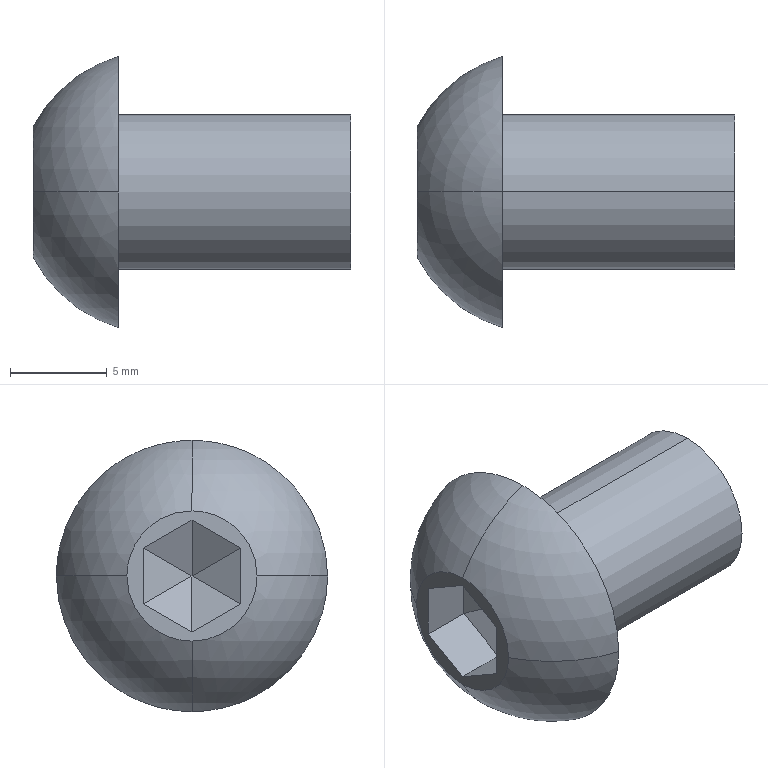Part | STEP file | PN_0030_Default<As Machined> | 1 solid | 21 faces | box 16.4 x 14 x 14 mm | volume 997.771 mm3 | plane 15 | sphere 4 | cylinder 2 | commonest cylinder face diameters 8 x2
STEP:
#1=CARTESIAN_POINT('',(0.,0.,-3.36));
#2=VERTEX_POINT('',#1);
#3=CARTESIAN_POINT('',(4.4,0.,-7.));
#4=VERTEX_POINT('',#3);
#5=CARTESIAN_POINT('',(6.485,0.,0.));
#6=DIRECTION('',(0.,-1.,0.));
#7=AXIS2_PLACEMENT_3D('',#5,#6,$);
#8=CIRCLE('',#7,7.304);
#9=EDGE_CURVE('',#2,#4,#8,.T.);
#10=ORIENTED_EDGE('',*,*,#9,.T.);
#11=CARTESIAN_POINT('',(4.4,-7.,0.));
#12=VERTEX_POINT('',#11);
#13=CARTESIAN_POINT('',(4.4,0.,-7.));
#14=CARTESIAN_POINT('',(4.4,-0.2377,-7.));
#15=CARTESIAN_POINT('',(4.4,-0.4753,-6.99));
#16=CARTESIAN_POINT('',(4.4,-0.7247,-6.969));
#17=CARTESIAN_POINT('',(4.4,-1.178,-6.914));
#18=CARTESIAN_POINT('',(4.4,-1.742,-6.786));
#19=CARTESIAN_POINT('',(4.4,-1.99,-6.72));
#20=CARTESIAN_POINT('',(4.4,-2.558,-6.536));
#21=CARTESIAN_POINT('',(4.4,-3.208,-6.239));
#22=CARTESIAN_POINT('',(4.4,-3.559,-6.049));
#23=CARTESIAN_POINT('',(4.4,-4.629,-5.356));
#24=CARTESIAN_POINT('',(4.4,-5.585,-4.372));
#25=CARTESIAN_POINT('',(4.4,-6.11,-3.596));
#26=CARTESIAN_POINT('',(4.4,-6.66,-2.408));
#27=CARTESIAN_POINT('',(4.4,-6.923,-1.138));
#28=CARTESIAN_POINT('',(4.4,-6.974,-0.7603));
#29=CARTESIAN_POINT('',(4.4,-7.,-0.3801));
#30=CARTESIAN_POINT('',(4.4,-7.,0.));
#31=B_SPLINE_CURVE_WITH_KNOTS('',5,(#13,#14,#15,#16,#17,#18,#19,#20,#21,#22,#23,#24,#25,#26,#27,#28,#29,#30),.UNSPECIFIED.,.F.,.U.,(6,3,3,3,3,6),(0.,4.329,7.196,10.306,16.762,19.45),.UNSPECIFIED.);
#32=EDGE_CURVE('',#4,#12,#31,.T.);
#33=ORIENTED_EDGE('',*,*,#32,.T.);
#34=CARTESIAN_POINT('',(0.,-3.36,0.));
#35=VERTEX_POINT('',#34);
#36=CARTESIAN_POINT('',(6.485,0.,0.));
#37=DIRECTION('',(0.,0.,-1.));
#38=AXIS2_PLACEMENT_3D('',#36,#37,$);
#39=CIRCLE('',#38,7.304);
#40=EDGE_CURVE('',#12,#35,#39,.T.);
#41=ORIENTED_EDGE('',*,*,#40,.T.);
#42=CARTESIAN_POINT('',(0.,0.,-3.36));
#43=CARTESIAN_POINT('',(0.,-0.6331,-3.36));
#44=CARTESIAN_POINT('',(0.,-1.266,-3.211));
#45=CARTESIAN_POINT('',(0.000000147,-1.873,-2.911));
#46=CARTESIAN_POINT('',(-0.000000088,-2.698,-2.185));
#47=CARTESIAN_POINT('',(0.000000053,-3.177,-1.204));
#48=CARTESIAN_POINT('',(0.,-3.299,-0.8106));
#49=CARTESIAN_POINT('',(0.,-3.36,-0.4053));
#50=CARTESIAN_POINT('',(0.,-3.36,0.));
#51=B_SPLINE_CURVE_WITH_KNOTS('',5,(#42,#43,#44,#45,#46,#47,#48,#49,#50),.UNSPECIFIED.,.F.,.U.,(6,3,6),(0.,4.768,7.633),.UNSPECIFIED.);
#52=EDGE_CURVE('',#2,#35,#51,.T.);
#53=ORIENTED_EDGE('',*,*,#52,.F.);
#54=EDGE_LOOP('',(#10,#33,#41,#53));
#55=FACE_OUTER_BOUND('',#54,.T.);
#56=CARTESIAN_POINT('',(6.485,0.,0.));
#57=DIRECTION('',(0.,0.,-1.));
#58=DIRECTION('',(0.,-1.,0.));
#59=AXIS2_PLACEMENT_3D('',#56,#57,#58);
#60=SPHERICAL_SURFACE('',#59,7.304);
#61=ADVANCED_FACE('',(#55),#60,.T.);
#62=ORIENTED_EDGE('',*,*,#9,.F.);
#63=CARTESIAN_POINT('',(0.,3.36,0.));
#64=VERTEX_POINT('',#63);
#65=CARTESIAN_POINT('',(0.,3.36,0.));
#66=CARTESIAN_POINT('',(0.,3.36,-0.3593));
#67=CARTESIAN_POINT('',(0.,3.312,-0.7187));
#68=CARTESIAN_POINT('',(-0.000000044,3.216,-1.07));
#69=CARTESIAN_POINT('',(0.000000044,2.93,-1.742));
#70=CARTESIAN_POINT('',(-0.000000045,2.479,-2.312));
#71=CARTESIAN_POINT('',(0.000000004,2.216,-2.564));
#72=CARTESIAN_POINT('',(-0.000000004,1.643,-2.983));
#73=CARTESIAN_POINT('',(0.000000004,0.9962,-3.236));
#74=CARTESIAN_POINT('',(0.,0.6671,-3.319));
#75=CARTESIAN_POINT('',(0.,0.3335,-3.36));
#76=CARTESIAN_POINT('',(0.,0.,-3.36));
#77=B_SPLINE_CURVE_WITH_KNOTS('',5,(#65,#66,#67,#68,#69,#70,#71,#72,#73,#74,#75,#76),.UNSPECIFIED.,.F.,.U.,(6,3,3,6),(0.,2.541,5.121,7.633),.UNSPECIFIED.);
#78=EDGE_CURVE('',#64,#2,#77,.T.);
#79=ORIENTED_EDGE('',*,*,#78,.F.);
#80=CARTESIAN_POINT('',(4.4,7.,0.));
#81=VERTEX_POINT('',#80);
#82=CARTESIAN_POINT('',(6.485,0.,0.));
#83=DIRECTION('',(0.,0.,-1.));
#84=AXIS2_PLACEMENT_3D('',#82,#83,$);
#85=CIRCLE('',#84,7.304);
#86=EDGE_CURVE('',#81,#64,#85,.F.);
#87=ORIENTED_EDGE('',*,*,#86,.F.);
#88=CARTESIAN_POINT('',(4.4,7.,0.));
#89=CARTESIAN_POINT('',(4.4,7.,-0.5217));
#90=CARTESIAN_POINT('',(4.4,6.951,-1.043));
#91=CARTESIAN_POINT('',(4.4,6.854,-1.556));
#92=CARTESIAN_POINT('',(4.4,6.568,-2.555));
#93=CARTESIAN_POINT('',(4.4,6.105,-3.484));
#94=CARTESIAN_POINT('',(4.4,5.83,-3.927));
#95=CARTESIAN_POINT('',(4.4,5.184,-4.778));
#96=CARTESIAN_POINT('',(4.4,4.402,-5.482));
#97=CARTESIAN_POINT('',(4.4,3.966,-5.803));
#98=CARTESIAN_POINT('',(4.4,3.252,-6.229));
#99=CARTESIAN_POINT('',(4.4,2.583,-6.515));
#100=CARTESIAN_POINT('',(4.4,2.338,-6.605));
#101=CARTESIAN_POINT('',(4.4,1.566,-6.853));
#102=CARTESIAN_POINT('',(4.4,0.9802,-6.945));
#103=CARTESIAN_POINT('',(4.4,0.6376,-6.982));
#104=CARTESIAN_POINT('',(4.4,0.3188,-7.));
#105=CARTESIAN_POINT('',(4.4,0.,-7.));
#106=B_SPLINE_CURVE_WITH_KNOTS('',5,(#88,#89,#90,#91,#92,#93,#94,#95,#96,#97,#98,#99,#100,#101,#102,#103,#104,#105),.UNSPECIFIED.,.F.,.U.,(6,3,3,3,3,6),(0.,3.689,7.378,11.242,13.675,19.481),.UNSPECIFIED.);
#107=EDGE_CURVE('',#81,#4,#106,.T.);
#108=ORIENTED_EDGE('',*,*,#107,.T.);
#109=EDGE_LOOP('',(#62,#79,#87,#108));
#110=FACE_OUTER_BOUND('',#109,.T.);
#111=CARTESIAN_POINT('',(6.485,0.,0.));
#112=DIRECTION('',(0.,0.,-1.));
#113=DIRECTION('',(-1.,0.,0.));
#114=AXIS2_PLACEMENT_3D('',#111,#112,#113);
#115=SPHERICAL_SURFACE('',#114,7.304);
#116=ADVANCED_FACE('',(#110),#115,.T.);
#117=ORIENTED_EDGE('',*,*,#32,.F.);
#118=ORIENTED_EDGE('',*,*,#107,.F.);
#119=CARTESIAN_POINT('',(4.4,0.,7.));
#120=VERTEX_POINT('',#119);
#121=CARTESIAN_POINT('',(4.4,0.,7.));
#122=CARTESIAN_POINT('',(4.4,0.3932,7.));
#123=CARTESIAN_POINT('',(4.4,0.7864,6.972));
#124=CARTESIAN_POINT('',(4.4,1.177,6.917));
#125=CARTESIAN_POINT('',(4.4,2.198,6.699));
#126=CARTESIAN_POINT('',(4.4,3.165,6.294));
#127=CARTESIAN_POINT('',(4.4,3.735,5.974));
#128=CARTESIAN_POINT('',(4.4,4.79,5.207));
#129=CARTESIAN_POINT('',(4.4,5.642,4.219));
#130=CARTESIAN_POINT('',(4.4,6.009,3.677));
#131=CARTESIAN_POINT('',(4.4,6.547,2.643));
#132=CARTESIAN_POINT('',(4.4,6.861,1.524));
#133=CARTESIAN_POINT('',(4.4,6.954,1.02));
#134=CARTESIAN_POINT('',(4.4,7.,0.5098));
#135=CARTESIAN_POINT('',(4.4,7.,0.));
#136=B_SPLINE_CURVE_WITH_KNOTS('',5,(#121,#122,#123,#124,#125,#126,#127,#128,#129,#130,#131,#132,#133,#134,#135),.UNSPECIFIED.,.F.,.U.,(6,3,3,3,6),(15.55,18.33,22.913,27.495,31.1),.UNSPECIFIED.);
#137=EDGE_CURVE('',#120,#81,#136,.T.);
#138=ORIENTED_EDGE('',*,*,#137,.F.);
#139=CARTESIAN_POINT('',(4.4,-7.,0.));
#140=CARTESIAN_POINT('',(4.4,-7.,0.6481));
#141=CARTESIAN_POINT('',(4.4,-6.925,1.296));
#142=CARTESIAN_POINT('',(4.4,-6.775,1.933));
#143=CARTESIAN_POINT('',(4.4,-6.33,3.159));
#144=CARTESIAN_POINT('',(4.4,-5.617,4.252));
#145=CARTESIAN_POINT('',(4.4,-5.199,4.755));
#146=CARTESIAN_POINT('',(4.4,-4.253,5.654));
#147=CARTESIAN_POINT('',(4.4,-3.127,6.313));
#148=CARTESIAN_POINT('',(4.4,-2.529,6.576));
#149=CARTESIAN_POINT('',(4.4,-1.659,6.842));
#150=CARTESIAN_POINT('',(4.4,-0.764,6.965));
#151=CARTESIAN_POINT('',(4.4,-0.5098,6.988));
#152=CARTESIAN_POINT('',(4.4,-0.2549,7.));
#153=CARTESIAN_POINT('',(4.4,0.,7.));
#154=B_SPLINE_CURVE_WITH_KNOTS('',5,(#139,#140,#141,#142,#143,#144,#145,#146,#147,#148,#149,#150,#151,#152,#153),.UNSPECIFIED.,.F.,.U.,(6,3,3,3,6),(0.,4.583,9.165,13.748,15.55),.UNSPECIFIED.);
#155=EDGE_CURVE('',#12,#120,#154,.T.);
#156=ORIENTED_EDGE('',*,*,#155,.F.);
#157=EDGE_LOOP('',(#117,#118,#138,#156));
#158=FACE_OUTER_BOUND('',#157,.T.);
#159=CARTESIAN_POINT('',(4.4,0.,4.));
#160=VERTEX_POINT('',#159);
#161=CARTESIAN_POINT('',(4.4,0.,-4.));
#162=VERTEX_POINT('',#161);
#163=CARTESIAN_POINT('',(4.4,0.,0.));
#164=DIRECTION('',(1.,0.,0.));
#165=AXIS2_PLACEMENT_3D('',#163,#164,$);
#166=CIRCLE('',#165,4.);
#167=EDGE_CURVE('',#160,#162,#166,.T.);
#168=ORIENTED_EDGE('',*,*,#167,.F.);
#169=CARTESIAN_POINT('',(4.4,0.,0.));
#170=DIRECTION('',(1.,0.,0.));
#171=AXIS2_PLACEMENT_3D('',#169,#170,$);
#172=CIRCLE('',#171,4.);
#173=EDGE_CURVE('',#162,#160,#172,.T.);
#174=ORIENTED_EDGE('',*,*,#173,.F.);
#175=EDGE_LOOP('',(#168,#174));
#176=FACE_BOUND('',#175,.T.);
#177=CARTESIAN_POINT('',(4.4,0.,0.));
#178=DIRECTION('',(1.,0.,0.));
#179=DIRECTION('',(0.,0.,-1.));
#180=AXIS2_PLACEMENT_3D('',#177,#178,#179);
#181=PLANE('',#180);
#182=ADVANCED_FACE('',(#158,#176),#181,.T.);
#183=CARTESIAN_POINT('',(0.,0.,3.36));
#184=VERTEX_POINT('',#183);
#185=CARTESIAN_POINT('',(6.485,0.,0.));
#186=DIRECTION('',(0.,-1.,0.));
#187=AXIS2_PLACEMENT_3D('',#185,#186,$);
#188=CIRCLE('',#187,7.304);
#189=EDGE_CURVE('',#120,#184,#188,.T.);
#190=ORIENTED_EDGE('',*,*,#189,.T.);
#191=CARTESIAN_POINT('',(0.,-3.36,0.));
#192=CARTESIAN_POINT('',(0.,-3.36,0.3593));
#193=CARTESIAN_POINT('',(0.,-3.312,0.7187));
#194=CARTESIAN_POINT('',(-0.000000044,-3.216,1.07));
#195=CARTESIAN_POINT('',(0.000000044,-2.93,1.742));
#196=CARTESIAN_POINT('',(-0.000000045,-2.479,2.312));
#197=CARTESIAN_POINT('',(0.000000004,-2.216,2.564));
#198=CARTESIAN_POINT('',(-0.000000004,-1.643,2.983));
#199=CARTESIAN_POINT('',(0.000000004,-0.9962,3.236));
#200=CARTESIAN_POINT('',(0.,-0.6671,3.319));
#201=CARTESIAN_POINT('',(0.,-0.3335,3.36));
#202=CARTESIAN_POINT('',(0.,0.,3.36));
#203=B_SPLINE_CURVE_WITH_KNOTS('',5,(#191,#192,#193,#194,#195,#196,#197,#198,#199,#200,#201,#202),.UNSPECIFIED.,.F.,.U.,(6,3,3,6),(0.,2.541,5.121,7.633),.UNSPECIFIED.);
#204=EDGE_CURVE('',#35,#184,#203,.T.);
#205=ORIENTED_EDGE('',*,*,#204,.F.);
#206=ORIENTED_EDGE('',*,*,#40,.F.);
#207=ORIENTED_EDGE('',*,*,#155,.T.);
#208=EDGE_LOOP('',(#190,#205,#206,#207));
#209=FACE_OUTER_BOUND('',#208,.T.);
#210=CARTESIAN_POINT('',(6.485,0.,0.));
#211=DIRECTION('',(0.,0.,-1.));
#212=DIRECTION('',(0.,-1.,0.));
#213=AXIS2_PLACEMENT_3D('',#210,#211,#212);
#214=SPHERICAL_SURFACE('',#213,7.304);
#215=ADVANCED_FACE('',(#209),#214,.T.);
#216=ORIENTED_EDGE('',*,*,#78,.T.);
#217=ORIENTED_EDGE('',*,*,#52,.T.);
#218=ORIENTED_EDGE('',*,*,#204,.T.);
#219=CARTESIAN_POINT('',(0.,0.,3.36));
#220=CARTESIAN_POINT('',(0.,0.02202,3.36));
#221=CARTESIAN_POINT('',(0.,0.04404,3.36));
#222=CARTESIAN_POINT('',(0.,0.06606,3.359));
#223=CARTESIAN_POINT('',(0.,0.4472,3.35));
#224=CARTESIAN_POINT('',(0.,0.8265,3.287));
#225=CARTESIAN_POINT('',(0.,1.174,3.179));
#226=CARTESIAN_POINT('',(0.,1.831,2.874));
#227=CARTESIAN_POINT('',(0.,2.386,2.407));
#228=CARTESIAN_POINT('',(0.,2.63,2.138));
#229=CARTESIAN_POINT('',(0.,3.015,1.577));
#230=CARTESIAN_POINT('',(0.,3.249,0.9397));
#231=CARTESIAN_POINT('',(0.,3.323,0.6303));
#232=CARTESIAN_POINT('',(0.,3.36,0.3152));
#233=CARTESIAN_POINT('',(0.,3.36,0.));
#234=B_SPLINE_CURVE_WITH_KNOTS('',5,(#219,#220,#221,#222,#223,#224,#225,#226,#227,#228,#229,#230,#231,#232,#233),.UNSPECIFIED.,.F.,.U.,(6,3,3,3,6),(7.464,7.62,10.16,12.699,14.928),.UNSPECIFIED.);
#235=EDGE_CURVE('',#184,#64,#234,.T.);
#236=ORIENTED_EDGE('',*,*,#235,.T.);
#237=EDGE_LOOP('',(#216,#217,#218,#236));
#238=FACE_OUTER_BOUND('',#237,.T.);
#239=CARTESIAN_POINT('',(0.,-2.5,-1.443));
#240=VERTEX_POINT('',#239);
#241=CARTESIAN_POINT('',(0.,0.,-2.887));
#242=VERTEX_POINT('',#241);
#243=CARTESIAN_POINT('',(0.,-1.25,-2.165));
#244=DIRECTION('',(0.,0.866,-0.5));
#245=VECTOR('',#244,1.);
#246=LINE('',#243,#245);
#247=EDGE_CURVE('',#240,#242,#246,.T.);
#248=ORIENTED_EDGE('',*,*,#247,.T.);
#249=CARTESIAN_POINT('',(0.,2.5,-1.443));
#250=VERTEX_POINT('',#249);
#251=CARTESIAN_POINT('',(0.,1.25,-2.165));
#252=DIRECTION('',(0.,0.866,0.5));
#253=VECTOR('',#252,1.);
#254=LINE('',#251,#253);
#255=EDGE_CURVE('',#242,#250,#254,.T.);
#256=ORIENTED_EDGE('',*,*,#255,.T.);
#257=CARTESIAN_POINT('',(0.,2.5,1.443));
#258=VERTEX_POINT('',#257);
#259=CARTESIAN_POINT('',(0.,2.5,0.));
#260=DIRECTION('',(0.,0.,1.));
#261=VECTOR('',#260,1.);
#262=LINE('',#259,#261);
#263=EDGE_CURVE('',#250,#258,#262,.T.);
#264=ORIENTED_EDGE('',*,*,#263,.T.);
#265=CARTESIAN_POINT('',(0.,0.,2.887));
#266=VERTEX_POINT('',#265);
#267=CARTESIAN_POINT('',(0.,1.25,2.165));
#268=DIRECTION('',(0.,-0.866,0.5));
#269=VECTOR('',#268,1.);
#270=LINE('',#267,#269);
#271=EDGE_CURVE('',#258,#266,#270,.T.);
#272=ORIENTED_EDGE('',*,*,#271,.T.);
#273=CARTESIAN_POINT('',(0.,-2.5,1.443));
#274=VERTEX_POINT('',#273);
#275=CARTESIAN_POINT('',(0.,-1.25,2.165));
#276=DIRECTION('',(0.,-0.866,-0.5));
#277=VECTOR('',#276,1.);
#278=LINE('',#275,#277);
#279=EDGE_CURVE('',#266,#274,#278,.T.);
#280=ORIENTED_EDGE('',*,*,#279,.T.);
#281=CARTESIAN_POINT('',(0.,-2.5,0.));
#282=DIRECTION('',(0.,0.,-1.));
#283=VECTOR('',#282,1.);
#284=LINE('',#281,#283);
#285=EDGE_CURVE('',#274,#240,#284,.T.);
#286=ORIENTED_EDGE('',*,*,#285,.T.);
#287=EDGE_LOOP('',(#248,#256,#264,#272,#280,#286));
#288=FACE_BOUND('',#287,.T.);
#289=CARTESIAN_POINT('',(0.,0.,0.));
#290=DIRECTION('',(1.,0.,0.));
#291=DIRECTION('',(0.,0.,-1.));
#292=AXIS2_PLACEMENT_3D('',#289,#290,#291);
#293=PLANE('',#292);
#294=ADVANCED_FACE('',(#238,#288),#293,.F.);
#295=ORIENTED_EDGE('',*,*,#189,.F.);
#296=ORIENTED_EDGE('',*,*,#137,.T.);
#297=ORIENTED_EDGE('',*,*,#86,.T.);
#298=ORIENTED_EDGE('',*,*,#235,.F.);
#299=EDGE_LOOP('',(#295,#296,#297,#298));
#300=FACE_OUTER_BOUND('',#299,.T.);
#301=CARTESIAN_POINT('',(6.485,0.,0.));
#302=DIRECTION('',(0.,0.,-1.));
#303=DIRECTION('',(-1.,0.,0.));
#304=AXIS2_PLACEMENT_3D('',#301,#302,#303);
#305=SPHERICAL_SURFACE('',#304,7.304);
#306=ADVANCED_FACE('',(#300),#305,.T.);
#307=CARTESIAN_POINT('',(16.4,0.,-4.));
#308=VERTEX_POINT('',#307);
#309=CARTESIAN_POINT('',(16.4,0.,-4.));
#310=DIRECTION('',(-1.,0.,0.));
#311=VECTOR('',#310,1.);
#312=LINE('',#309,#311);
#313=EDGE_CURVE('',#308,#162,#312,.T.);
#314=ORIENTED_EDGE('',*,*,#313,.F.);
#315=CARTESIAN_POINT('',(16.4,0.,4.));
#316=VERTEX_POINT('',#315);
#317=CARTESIAN_POINT('',(16.4,0.,0.));
#318=DIRECTION('',(-1.,0.,0.));
#319=AXIS2_PLACEMENT_3D('',#317,#318,$);
#320=CIRCLE('',#319,4.);
#321=EDGE_CURVE('',#316,#308,#320,.F.);
#322=ORIENTED_EDGE('',*,*,#321,.F.);
#323=CARTESIAN_POINT('',(16.4,0.,4.));
#324=DIRECTION('',(-1.,0.,0.));
#325=VECTOR('',#324,1.);
#326=LINE('',#323,#325);
#327=EDGE_CURVE('',#316,#160,#326,.T.);
#328=ORIENTED_EDGE('',*,*,#327,.T.);
#329=ORIENTED_EDGE('',*,*,#167,.T.);
#330=EDGE_LOOP('',(#314,#322,#328,#329));
#331=FACE_OUTER_BOUND('',#330,.T.);
#332=CARTESIAN_POINT('',(16.4,0.,0.));
#333=DIRECTION('',(-1.,0.,0.));
#334=DIRECTION('',(0.,0.,-1.));
#335=AXIS2_PLACEMENT_3D('',#332,#333,#334);
#336=CYLINDRICAL_SURFACE('',#335,4.);
#337=ADVANCED_FACE('',(#331),#336,.T.);
#338=CARTESIAN_POINT('',(16.4,0.,0.));
#339=DIRECTION('',(-1.,0.,0.));
#340=AXIS2_PLACEMENT_3D('',#338,#339,$);
#341=CIRCLE('',#340,4.);
#342=EDGE_CURVE('',#308,#316,#341,.F.);
#343=ORIENTED_EDGE('',*,*,#342,.F.);
#344=ORIENTED_EDGE('',*,*,#313,.T.);
#345=ORIENTED_EDGE('',*,*,#173,.T.);
#346=ORIENTED_EDGE('',*,*,#327,.F.);
#347=EDGE_LOOP('',(#343,#344,#345,#346));
#348=FACE_OUTER_BOUND('',#347,.T.);
#349=CARTESIAN_POINT('',(16.4,0.,0.));
#350=DIRECTION('',(-1.,0.,0.));
#351=DIRECTION('',(0.,0.,1.));
#352=AXIS2_PLACEMENT_3D('',#349,#350,#351);
#353=CYLINDRICAL_SURFACE('',#352,4.);
#354=ADVANCED_FACE('',(#348),#353,.T.);
#355=ORIENTED_EDGE('',*,*,#247,.F.);
#356=CARTESIAN_POINT('',(2.6,-2.5,-1.443));
#357=VERTEX_POINT('',#356);
#358=CARTESIAN_POINT('',(1.3,-2.5,-1.443));
#359=DIRECTION('',(-1.,0.,0.));
#360=VECTOR('',#359,1.);
#361=LINE('',#358,#360);
#362=EDGE_CURVE('',#357,#240,#361,.T.);
#363=ORIENTED_EDGE('',*,*,#362,.F.);
#364=CARTESIAN_POINT('',(2.6,0.,-2.887));
#365=VERTEX_POINT('',#364);
#366=CARTESIAN_POINT('',(2.6,-1.25,-2.165));
#367=DIRECTION('',(0.,0.866,-0.5));
#368=VECTOR('',#367,1.);
#369=LINE('',#366,#368);
#370=EDGE_CURVE('',#357,#365,#369,.T.);
#371=ORIENTED_EDGE('',*,*,#370,.T.);
#372=CARTESIAN_POINT('',(1.3,0.,-2.887));
#373=DIRECTION('',(-1.,0.,0.));
#374=VECTOR('',#373,1.);
#375=LINE('',#372,#374);
#376=EDGE_CURVE('',#365,#242,#375,.T.);
#377=ORIENTED_EDGE('',*,*,#376,.T.);
#378=EDGE_LOOP('',(#355,#363,#371,#377));
#379=FACE_OUTER_BOUND('',#378,.T.);
#380=CARTESIAN_POINT('',(2.6,-2.5,-1.443));
#381=DIRECTION('',(0.,0.5,0.866));
#382=DIRECTION('',(0.,-0.866,0.5));
#383=AXIS2_PLACEMENT_3D('',#380,#381,#382);
#384=PLANE('',#383);
#385=ADVANCED_FACE('',(#379),#384,.T.);
#386=ORIENTED_EDGE('',*,*,#255,.F.);
#387=ORIENTED_EDGE('',*,*,#376,.F.);
#388=CARTESIAN_POINT('',(2.6,2.5,-1.443));
#389=VERTEX_POINT('',#388);
#390=CARTESIAN_POINT('',(2.6,1.25,-2.165));
#391=DIRECTION('',(0.,0.866,0.5));
#392=VECTOR('',#391,1.);
#393=LINE('',#390,#392);
#394=EDGE_CURVE('',#365,#389,#393,.T.);
#395=ORIENTED_EDGE('',*,*,#394,.T.);
#396=CARTESIAN_POINT('',(1.3,2.5,-1.443));
#397=DIRECTION('',(-1.,0.,0.));
#398=VECTOR('',#397,1.);
#399=LINE('',#396,#398);
#400=EDGE_CURVE('',#389,#250,#399,.T.);
#401=ORIENTED_EDGE('',*,*,#400,.T.);
#402=EDGE_LOOP('',(#386,#387,#395,#401));
#403=FACE_OUTER_BOUND('',#402,.T.);
#404=CARTESIAN_POINT('',(2.6,0.,-2.887));
#405=DIRECTION('',(0.,-0.5,0.866));
#406=DIRECTION('',(0.,-0.866,-0.5));
#407=AXIS2_PLACEMENT_3D('',#404,#405,#406);
#408=PLANE('',#407);
#409=ADVANCED_FACE('',(#403),#408,.T.);
#410=ORIENTED_EDGE('',*,*,#263,.F.);
#411=ORIENTED_EDGE('',*,*,#400,.F.);
#412=CARTESIAN_POINT('',(2.6,2.5,1.443));
#413=VERTEX_POINT('',#412);
#414=CARTESIAN_POINT('',(2.6,2.5,0.));
#415=DIRECTION('',(0.,0.,1.));
#416=VECTOR('',#415,1.);
#417=LINE('',#414,#416);
#418=EDGE_CURVE('',#389,#413,#417,.T.);
#419=ORIENTED_EDGE('',*,*,#418,.T.);
#420=CARTESIAN_POINT('',(1.3,2.5,1.443));
#421=DIRECTION('',(-1.,0.,0.));
#422=VECTOR('',#421,1.);
#423=LINE('',#420,#422);
#424=EDGE_CURVE('',#413,#258,#423,.T.);
#425=ORIENTED_EDGE('',*,*,#424,.T.);
#426=EDGE_LOOP('',(#410,#411,#419,#425));
#427=FACE_OUTER_BOUND('',#426,.T.);
#428=CARTESIAN_POINT('',(2.6,2.5,-1.443));
#429=DIRECTION('',(0.,-1.,0.));
#430=DIRECTION('',(0.,0.,-1.));
#431=AXIS2_PLACEMENT_3D('',#428,#429,#430);
#432=PLANE('',#431);
#433=ADVANCED_FACE('',(#427),#432,.T.);
#434=ORIENTED_EDGE('',*,*,#271,.F.);
#435=ORIENTED_EDGE('',*,*,#424,.F.);
#436=CARTESIAN_POINT('',(2.6,0.,2.887));
#437=VERTEX_POINT('',#436);
#438=CARTESIAN_POINT('',(2.6,1.25,2.165));
#439=DIRECTION('',(0.,-0.866,0.5));
#440=VECTOR('',#439,1.);
#441=LINE('',#438,#440);
#442=EDGE_CURVE('',#413,#437,#441,.T.);
#443=ORIENTED_EDGE('',*,*,#442,.T.);
#444=CARTESIAN_POINT('',(1.3,0.,2.887));
#445=DIRECTION('',(-1.,0.,0.));
#446=VECTOR('',#445,1.);
#447=LINE('',#444,#446);
#448=EDGE_CURVE('',#437,#266,#447,.T.);
#449=ORIENTED_EDGE('',*,*,#448,.T.);
#450=EDGE_LOOP('',(#434,#435,#443,#449));
#451=FACE_OUTER_BOUND('',#450,.T.);
#452=CARTESIAN_POINT('',(2.6,2.5,1.443));
#453=DIRECTION('',(0.,-0.5,-0.866));
#454=DIRECTION('',(0.,0.866,-0.5));
#455=AXIS2_PLACEMENT_3D('',#452,#453,#454);
#456=PLANE('',#455);
#457=ADVANCED_FACE('',(#451),#456,.T.);
#458=ORIENTED_EDGE('',*,*,#279,.F.);
#459=ORIENTED_EDGE('',*,*,#448,.F.);
#460=CARTESIAN_POINT('',(2.6,-2.5,1.443));
#461=VERTEX_POINT('',#460);
#462=CARTESIAN_POINT('',(2.6,-1.25,2.165));
#463=DIRECTION('',(0.,-0.866,-0.5));
#464=VECTOR('',#463,1.);
#465=LINE('',#462,#464);
#466=EDGE_CURVE('',#437,#461,#465,.T.);
#467=ORIENTED_EDGE('',*,*,#466,.T.);
#468=CARTESIAN_POINT('',(1.3,-2.5,1.443));
#469=DIRECTION('',(-1.,0.,0.));
#470=VECTOR('',#469,1.);
#471=LINE('',#468,#470);
#472=EDGE_CURVE('',#461,#274,#471,.T.);
#473=ORIENTED_EDGE('',*,*,#472,.T.);
#474=EDGE_LOOP('',(#458,#459,#467,#473));
#475=FACE_OUTER_BOUND('',#474,.T.);
#476=CARTESIAN_POINT('',(2.6,0.,2.887));
#477=DIRECTION('',(0.,0.5,-0.866));
#478=DIRECTION('',(0.,0.866,0.5));
#479=AXIS2_PLACEMENT_3D('',#476,#477,#478);
#480=PLANE('',#479);
#481=ADVANCED_FACE('',(#475),#480,.T.);
#482=ORIENTED_EDGE('',*,*,#285,.F.);
#483=ORIENTED_EDGE('',*,*,#472,.F.);
#484=CARTESIAN_POINT('',(2.6,-2.5,0.));
#485=DIRECTION('',(0.,0.,-1.));
#486=VECTOR('',#485,1.);
#487=LINE('',#484,#486);
#488=EDGE_CURVE('',#461,#357,#487,.T.);
#489=ORIENTED_EDGE('',*,*,#488,.T.);
#490=ORIENTED_EDGE('',*,*,#362,.T.);
#491=EDGE_LOOP('',(#482,#483,#489,#490));
#492=FACE_OUTER_BOUND('',#491,.T.);
#493=CARTESIAN_POINT('',(2.6,-2.5,1.443));
#494=DIRECTION('',(0.,1.,0.));
#495=DIRECTION('',(0.,0.,1.));
#496=AXIS2_PLACEMENT_3D('',#493,#494,#495);
#497=PLANE('',#496);
#498=ADVANCED_FACE('',(#492),#497,.T.);
#499=ORIENTED_EDGE('',*,*,#321,.T.);
#500=ORIENTED_EDGE('',*,*,#342,.T.);
#501=EDGE_LOOP('',(#499,#500));
#502=FACE_OUTER_BOUND('',#501,.T.);
#503=CARTESIAN_POINT('',(16.4,0.,0.));
#504=DIRECTION('',(1.,0.,0.));
#505=DIRECTION('',(0.,0.,-1.));
#506=AXIS2_PLACEMENT_3D('',#503,#504,#505);
#507=PLANE('',#506);
#508=ADVANCED_FACE('',(#502),#507,.T.);
#509=ORIENTED_EDGE('',*,*,#370,.F.);
#510=CARTESIAN_POINT('',(4.043,0.,-0.000000001));
#511=VERTEX_POINT('',#510);
#512=CARTESIAN_POINT('',(3.322,-1.25,-0.7217));
#513=DIRECTION('',(-0.4472,-0.7746,-0.4472));
#514=VECTOR('',#513,1.);
#515=LINE('',#512,#514);
#516=EDGE_CURVE('',#511,#357,#515,.T.);
#517=ORIENTED_EDGE('',*,*,#516,.F.);
#518=CARTESIAN_POINT('',(3.322,0.,-1.443));
#519=DIRECTION('',(-0.4472,0.,-0.8944));
#520=VECTOR('',#519,1.);
#521=LINE('',#518,#520);
#522=EDGE_CURVE('',#511,#365,#521,.T.);
#523=ORIENTED_EDGE('',*,*,#522,.T.);
#524=EDGE_LOOP('',(#509,#517,#523));
#525=FACE_OUTER_BOUND('',#524,.T.);
#526=CARTESIAN_POINT('',(2.6,-2.5,-1.443));
#527=DIRECTION('',(0.866,-0.25,-0.433));
#528=DIRECTION('',(-0.4472,0.,-0.8944));
#529=AXIS2_PLACEMENT_3D('',#526,#527,#528);
#530=PLANE('',#529);
#531=ADVANCED_FACE('',(#525),#530,.F.);
#532=ORIENTED_EDGE('',*,*,#394,.F.);
#533=ORIENTED_EDGE('',*,*,#522,.F.);
#534=CARTESIAN_POINT('',(3.322,1.25,-0.7217));
#535=DIRECTION('',(-0.4472,0.7746,-0.4472));
#536=VECTOR('',#535,1.);
#537=LINE('',#534,#536);
#538=EDGE_CURVE('',#511,#389,#537,.T.);
#539=ORIENTED_EDGE('',*,*,#538,.T.);
#540=EDGE_LOOP('',(#532,#533,#539));
#541=FACE_OUTER_BOUND('',#540,.T.);
#542=CARTESIAN_POINT('',(2.6,0.,-2.887));
#543=DIRECTION('',(0.866,0.25,-0.433));
#544=DIRECTION('',(-0.4472,0.,-0.8944));
#545=AXIS2_PLACEMENT_3D('',#542,#543,#544);
#546=PLANE('',#545);
#547=ADVANCED_FACE('',(#541),#546,.F.);
#548=ORIENTED_EDGE('',*,*,#418,.F.);
#549=ORIENTED_EDGE('',*,*,#538,.F.);
#550=CARTESIAN_POINT('',(3.322,1.25,0.7217));
#551=DIRECTION('',(-0.4472,0.7746,0.4472));
#552=VECTOR('',#551,1.);
#553=LINE('',#550,#552);
#554=EDGE_CURVE('',#511,#413,#553,.T.);
#555=ORIENTED_EDGE('',*,*,#554,.T.);
#556=EDGE_LOOP('',(#548,#549,#555));
#557=FACE_OUTER_BOUND('',#556,.T.);
#558=CARTESIAN_POINT('',(2.6,2.5,-1.443));
#559=DIRECTION('',(0.866,0.5,0.));
#560=DIRECTION('',(-0.5,0.866,0.));
#561=AXIS2_PLACEMENT_3D('',#558,#559,#560);
#562=PLANE('',#561);
#563=ADVANCED_FACE('',(#557),#562,.F.);
#564=ORIENTED_EDGE('',*,*,#442,.F.);
#565=ORIENTED_EDGE('',*,*,#554,.F.);
#566=CARTESIAN_POINT('',(3.322,0.,1.443));
#567=DIRECTION('',(-0.4472,0.,0.8944));
#568=VECTOR('',#567,1.);
#569=LINE('',#566,#568);
#570=EDGE_CURVE('',#511,#437,#569,.T.);
#571=ORIENTED_EDGE('',*,*,#570,.T.);
#572=EDGE_LOOP('',(#564,#565,#571));
#573=FACE_OUTER_BOUND('',#572,.T.);
#574=CARTESIAN_POINT('',(2.6,2.5,1.443));
#575=DIRECTION('',(0.866,0.25,0.433));
#576=DIRECTION('',(0.4472,0.,-0.8944));
#577=AXIS2_PLACEMENT_3D('',#574,#575,#576);
#578=PLANE('',#577);
#579=ADVANCED_FACE('',(#573),#578,.F.);
#580=ORIENTED_EDGE('',*,*,#466,.F.);
#581=ORIENTED_EDGE('',*,*,#570,.F.);
#582=CARTESIAN_POINT('',(3.322,-1.25,0.7217));
#583=DIRECTION('',(-0.4472,-0.7746,0.4472));
#584=VECTOR('',#583,1.);
#585=LINE('',#582,#584);
#586=EDGE_CURVE('',#511,#461,#585,.T.);
#587=ORIENTED_EDGE('',*,*,#586,.T.);
#588=EDGE_LOOP('',(#580,#581,#587));
#589=FACE_OUTER_BOUND('',#588,.T.);
#590=CARTESIAN_POINT('',(2.6,0.,2.887));
#591=DIRECTION('',(0.866,-0.25,0.433));
#592=DIRECTION('',(0.4472,0.,-0.8944));
#593=AXIS2_PLACEMENT_3D('',#590,#591,#592);
#594=PLANE('',#593);
#595=ADVANCED_FACE('',(#589),#594,.F.);
#596=ORIENTED_EDGE('',*,*,#488,.F.);
#597=ORIENTED_EDGE('',*,*,#586,.F.);
#598=ORIENTED_EDGE('',*,*,#516,.T.);
#599=EDGE_LOOP('',(#596,#597,#598));
#600=FACE_OUTER_BOUND('',#599,.T.);
#601=CARTESIAN_POINT('',(2.6,-2.5,1.443));
#602=DIRECTION('',(0.866,-0.5,0.));
#603=DIRECTION('',(0.5,0.866,0.));
#604=AXIS2_PLACEMENT_3D('',#601,#602,#603);
#605=PLANE('',#604);
#606=ADVANCED_FACE('',(#600),#605,.F.);
#607=CLOSED_SHELL('',(#61,#116,#182,#215,#294,#306,#337,#354,#385,#409,#433,#457,#481,#498,#508,#531,#547,#563,#579,#595,#606));
#608=MANIFOLD_SOLID_BREP('',#607);
#609=(LENGTH_UNIT()NAMED_UNIT(*)SI_UNIT(.MILLI.,.METRE.));
#610=UNCERTAINTY_MEASURE_WITH_UNIT(LENGTH_MEASURE(0.005),#609,'','');
#611=(NAMED_UNIT(*)PLANE_ANGLE_UNIT()SI_UNIT($,.RADIAN.));
#612=(NAMED_UNIT(*)SI_UNIT($,.STERADIAN.)SOLID_ANGLE_UNIT());
#613=(GEOMETRIC_REPRESENTATION_CONTEXT(3)GLOBAL_UNCERTAINTY_ASSIGNED_CONTEXT((#610))GLOBAL_UNIT_ASSIGNED_CONTEXT((#609,#611,#612))REPRESENTATION_CONTEXT('',''));
#614=ADVANCED_BREP_SHAPE_REPRESENTATION('',(#608),#613);